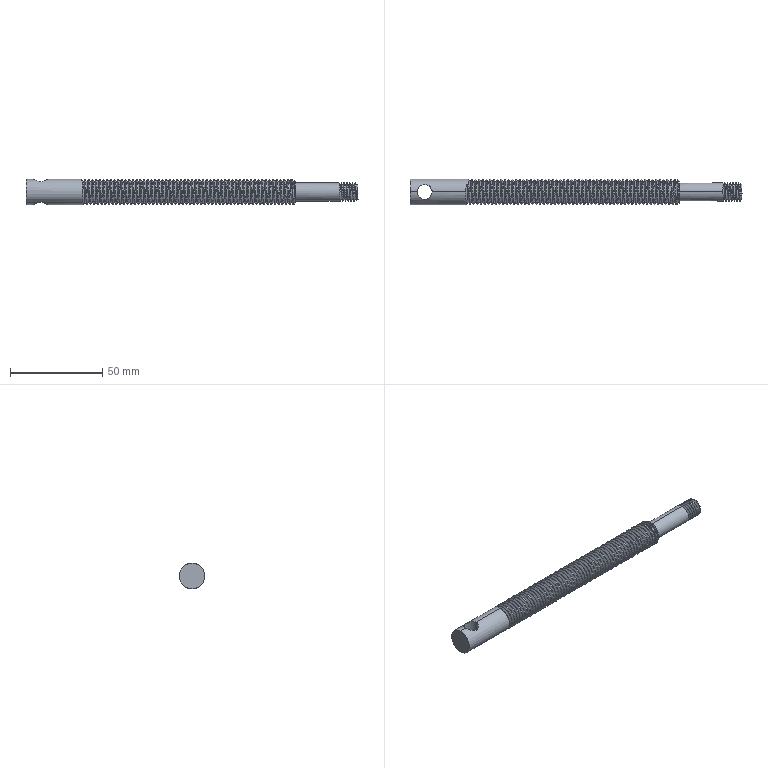Part | SolidWorks | features ICE 3, Chamfer 2, Helix 2, SweepCut 2, Revolution 1 | 1 solid | 156 faces | box 180 x 13.8 x 13.8 mm | volume 20623 mm3 | cylinder 135 | plane 9 | cone 6 | spline 6 | commonest cylinder face diameters 13.8 x116 9.8 x13 0.2 x2 0.4 x2 8 x2